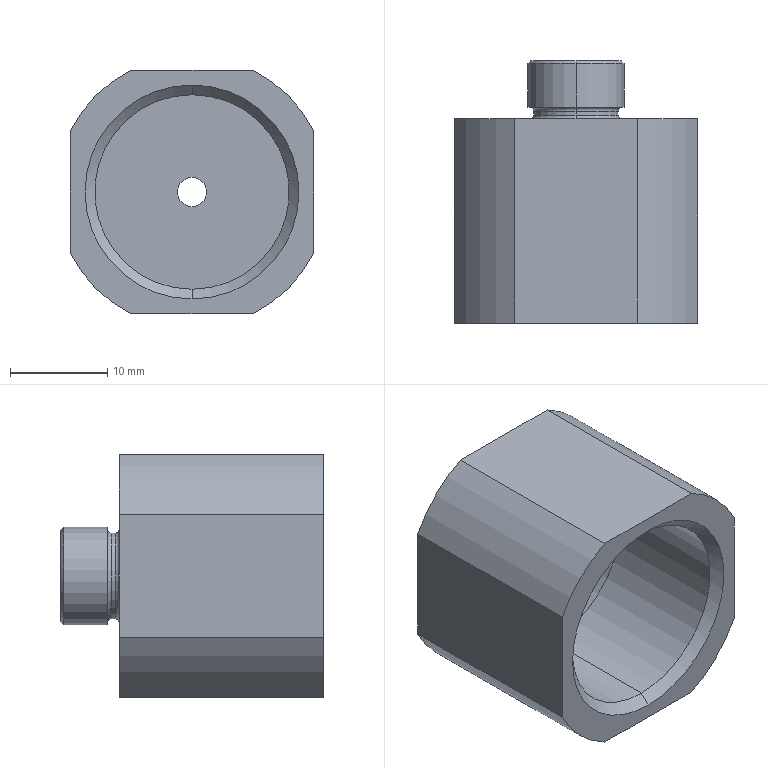Part | SolidWorks | features ICE 4, Chamfer 2, Fillet 1, Revolution 1 | 1 solid | 32 faces | box 25 x 27 x 25 mm | volume 6496 mm3 | cylinder 14 | plane 10 | cone 4 | torus 4 | commonest cylinder face diameters 28 x4 3 x2 8.8 x2 10 x2 20 x2 20.5 x2
STEP:
#1=CARTESIAN_POINT('',(0.,1.,10.));
#2=VERTEX_POINT('',#1);
#3=CARTESIAN_POINT('',(0.,1.,-10.));
#4=VERTEX_POINT('',#3);
#5=CARTESIAN_POINT('',(0.,1.,0.));
#6=DIRECTION('',(0.,-1.,0.));
#7=DIRECTION('',(0.,0.,-1.));
#8=AXIS2_PLACEMENT_3D('',#5,#6,#7);
#9=CIRCLE('',#8,10.);
#10=EDGE_CURVE('',#2,#4,#9,.T.);
#11=ORIENTED_EDGE('',*,*,#10,.F.);
#12=CARTESIAN_POINT('',(0.,0.,11.));
#13=VERTEX_POINT('',#12);
#14=CARTESIAN_POINT('',(0.,1.,10.));
#15=DIRECTION('',(0.,-0.7071,0.7071));
#16=VECTOR('',#15,1000.);
#17=LINE('',#14,#16);
#18=EDGE_CURVE('',#2,#13,#17,.T.);
#19=ORIENTED_EDGE('',*,*,#18,.T.);
#20=CARTESIAN_POINT('',(0.,0.,-11.));
#21=VERTEX_POINT('',#20);
#22=CARTESIAN_POINT('',(0.,0.,0.));
#23=DIRECTION('',(0.,1.,0.));
#24=DIRECTION('',(0.,0.,-1.));
#25=AXIS2_PLACEMENT_3D('',#22,#23,#24);
#26=CIRCLE('',#25,11.);
#27=EDGE_CURVE('',#21,#13,#26,.T.);
#28=ORIENTED_EDGE('',*,*,#27,.F.);
#29=CARTESIAN_POINT('',(0.,1.,-10.));
#30=DIRECTION('',(0.,-0.7071,-0.7071));
#31=VECTOR('',#30,1000.);
#32=LINE('',#29,#31);
#33=EDGE_CURVE('',#4,#21,#32,.T.);
#34=ORIENTED_EDGE('',*,*,#33,.F.);
#35=EDGE_LOOP('',(#11,#19,#28,#34));
#36=FACE_OUTER_BOUND('',#35,.T.);
#37=CARTESIAN_POINT('',(0.,1.,0.));
#38=DIRECTION('',(0.,-1.,0.));
#39=DIRECTION('',(0.,0.,-1.));
#40=AXIS2_PLACEMENT_3D('',#37,#38,#39);
#41=CONICAL_SURFACE('',#40,10.,0.7854);
#42=ADVANCED_FACE('',(#36),#41,.F.);
#43=CARTESIAN_POINT('',(0.,27.,4.7));
#44=VERTEX_POINT('',#43);
#45=CARTESIAN_POINT('',(0.,27.,-4.7));
#46=VERTEX_POINT('',#45);
#47=CARTESIAN_POINT('',(0.,27.,0.));
#48=DIRECTION('',(0.,1.,0.));
#49=DIRECTION('',(0.,0.,1.));
#50=AXIS2_PLACEMENT_3D('',#47,#48,#49);
#51=CIRCLE('',#50,4.7);
#52=EDGE_CURVE('',#44,#46,#51,.T.);
#53=ORIENTED_EDGE('',*,*,#52,.F.);
#54=CARTESIAN_POINT('',(0.,26.7,5.));
#55=VERTEX_POINT('',#54);
#56=CARTESIAN_POINT('',(0.,27.,4.7));
#57=DIRECTION('',(0.,-0.7071,0.7071));
#58=VECTOR('',#57,1000.);
#59=LINE('',#56,#58);
#60=EDGE_CURVE('',#44,#55,#59,.T.);
#61=ORIENTED_EDGE('',*,*,#60,.T.);
#62=CARTESIAN_POINT('',(0.,26.7,-5.));
#63=VERTEX_POINT('',#62);
#64=CARTESIAN_POINT('',(0.,26.7,0.));
#65=DIRECTION('',(0.,-1.,0.));
#66=DIRECTION('',(0.,0.,1.));
#67=AXIS2_PLACEMENT_3D('',#64,#65,#66);
#68=CIRCLE('',#67,5.);
#69=EDGE_CURVE('',#63,#55,#68,.T.);
#70=ORIENTED_EDGE('',*,*,#69,.F.);
#71=CARTESIAN_POINT('',(0.,27.,-4.7));
#72=DIRECTION('',(0.,-0.7071,-0.7071));
#73=VECTOR('',#72,1000.);
#74=LINE('',#71,#73);
#75=EDGE_CURVE('',#46,#63,#74,.T.);
#76=ORIENTED_EDGE('',*,*,#75,.F.);
#77=EDGE_LOOP('',(#53,#61,#70,#76));
#78=FACE_OUTER_BOUND('',#77,.T.);
#79=CARTESIAN_POINT('',(0.,27.,0.));
#80=DIRECTION('',(0.,-1.,0.));
#81=DIRECTION('',(0.,0.,-1.));
#82=AXIS2_PLACEMENT_3D('',#79,#80,#81);
#83=CONICAL_SURFACE('',#82,4.7,0.7854);
#84=ADVANCED_FACE('',(#78),#83,.T.);
#85=CARTESIAN_POINT('',(0.,27.,-1.5));
#86=VERTEX_POINT('',#85);
#87=CARTESIAN_POINT('',(0.,27.,1.5));
#88=VERTEX_POINT('',#87);
#89=CARTESIAN_POINT('',(0.,27.,0.));
#90=DIRECTION('',(0.,1.,0.));
#91=DIRECTION('',(0.,0.,1.));
#92=AXIS2_PLACEMENT_3D('',#89,#90,#91);
#93=CIRCLE('',#92,1.5);
#94=EDGE_CURVE('',#86,#88,#93,.T.);
#95=ORIENTED_EDGE('',*,*,#94,.T.);
#96=CARTESIAN_POINT('',(0.,18.,1.5));
#97=VERTEX_POINT('',#96);
#98=CARTESIAN_POINT('',(0.,108.,1.5));
#99=DIRECTION('',(0.,-1.,0.));
#100=VECTOR('',#99,1000.);
#101=LINE('',#98,#100);
#102=EDGE_CURVE('',#88,#97,#101,.T.);
#103=ORIENTED_EDGE('',*,*,#102,.T.);
#104=CARTESIAN_POINT('',(0.,18.,-1.5));
#105=VERTEX_POINT('',#104);
#106=CARTESIAN_POINT('',(0.,18.,0.));
#107=DIRECTION('',(0.,-1.,0.));
#108=DIRECTION('',(0.,0.,-1.));
#109=AXIS2_PLACEMENT_3D('',#106,#107,#108);
#110=CIRCLE('',#109,1.5);
#111=EDGE_CURVE('',#97,#105,#110,.T.);
#112=ORIENTED_EDGE('',*,*,#111,.T.);
#113=CARTESIAN_POINT('',(0.,108.,-1.5));
#114=DIRECTION('',(0.,-1.,0.));
#115=VECTOR('',#114,1000.);
#116=LINE('',#113,#115);
#117=EDGE_CURVE('',#86,#105,#116,.T.);
#118=ORIENTED_EDGE('',*,*,#117,.F.);
#119=EDGE_LOOP('',(#95,#103,#112,#118));
#120=FACE_OUTER_BOUND('',#119,.T.);
#121=CARTESIAN_POINT('',(0.,108.,0.));
#122=DIRECTION('',(0.,-1.,0.));
#123=DIRECTION('',(0.,0.,-1.));
#124=AXIS2_PLACEMENT_3D('',#121,#122,#123);
#125=CYLINDRICAL_SURFACE('',#124,1.5);
#126=ADVANCED_FACE('',(#120),#125,.F.);
#127=CARTESIAN_POINT('',(0.,18.,10.25));
#128=VERTEX_POINT('',#127);
#129=CARTESIAN_POINT('',(0.,18.,-10.25));
#130=VERTEX_POINT('',#129);
#131=CARTESIAN_POINT('',(0.,18.,0.));
#132=DIRECTION('',(0.,-1.,0.));
#133=DIRECTION('',(0.,0.,-1.));
#134=AXIS2_PLACEMENT_3D('',#131,#132,#133);
#135=CIRCLE('',#134,10.25);
#136=EDGE_CURVE('',#128,#130,#135,.T.);
#137=ORIENTED_EDGE('',*,*,#136,.F.);
#138=CARTESIAN_POINT('',(0.,14.,10.25));
#139=VERTEX_POINT('',#138);
#140=CARTESIAN_POINT('',(0.,18.,10.25));
#141=DIRECTION('',(0.,-1.,0.));
#142=VECTOR('',#141,1000.);
#143=LINE('',#140,#142);
#144=EDGE_CURVE('',#128,#139,#143,.T.);
#145=ORIENTED_EDGE('',*,*,#144,.T.);
#146=CARTESIAN_POINT('',(0.,14.,-10.25));
#147=VERTEX_POINT('',#146);
#148=CARTESIAN_POINT('',(0.,14.,0.));
#149=DIRECTION('',(0.,-1.,0.));
#150=DIRECTION('',(0.,0.,-1.));
#151=AXIS2_PLACEMENT_3D('',#148,#149,#150);
#152=CIRCLE('',#151,10.25);
#153=EDGE_CURVE('',#139,#147,#152,.T.);
#154=ORIENTED_EDGE('',*,*,#153,.T.);
#155=CARTESIAN_POINT('',(0.,18.,-10.25));
#156=DIRECTION('',(0.,-1.,0.));
#157=VECTOR('',#156,1000.);
#158=LINE('',#155,#157);
#159=EDGE_CURVE('',#130,#147,#158,.T.);
#160=ORIENTED_EDGE('',*,*,#159,.F.);
#161=EDGE_LOOP('',(#137,#145,#154,#160));
#162=FACE_OUTER_BOUND('',#161,.T.);
#163=CARTESIAN_POINT('',(0.,18.,0.));
#164=DIRECTION('',(0.,-1.,0.));
#165=DIRECTION('',(0.,0.,-1.));
#166=AXIS2_PLACEMENT_3D('',#163,#164,#165);
#167=CYLINDRICAL_SURFACE('',#166,10.25);
#168=ADVANCED_FACE('',(#162),#167,.F.);
#169=CARTESIAN_POINT('',(0.,14.,10.));
#170=VERTEX_POINT('',#169);
#171=CARTESIAN_POINT('',(0.,14.,-10.));
#172=VERTEX_POINT('',#171);
#173=CARTESIAN_POINT('',(0.,14.,0.));
#174=DIRECTION('',(0.,-1.,0.));
#175=DIRECTION('',(0.,0.,-1.));
#176=AXIS2_PLACEMENT_3D('',#173,#174,#175);
#177=CIRCLE('',#176,10.);
#178=EDGE_CURVE('',#170,#172,#177,.T.);
#179=ORIENTED_EDGE('',*,*,#178,.F.);
#180=CARTESIAN_POINT('',(0.,14.,10.));
#181=DIRECTION('',(0.,-1.,0.));
#182=VECTOR('',#181,1000.);
#183=LINE('',#180,#182);
#184=EDGE_CURVE('',#170,#2,#183,.T.);
#185=ORIENTED_EDGE('',*,*,#184,.T.);
#186=ORIENTED_EDGE('',*,*,#10,.T.);
#187=CARTESIAN_POINT('',(0.,14.,-10.));
#188=DIRECTION('',(0.,-1.,0.));
#189=VECTOR('',#188,1000.);
#190=LINE('',#187,#189);
#191=EDGE_CURVE('',#172,#4,#190,.T.);
#192=ORIENTED_EDGE('',*,*,#191,.F.);
#193=EDGE_LOOP('',(#179,#185,#186,#192));
#194=FACE_OUTER_BOUND('',#193,.T.);
#195=CARTESIAN_POINT('',(0.,14.,0.));
#196=DIRECTION('',(0.,-1.,0.));
#197=DIRECTION('',(0.,0.,-1.));
#198=AXIS2_PLACEMENT_3D('',#195,#196,#197);
#199=CYLINDRICAL_SURFACE('',#198,10.);
#200=ADVANCED_FACE('',(#194),#199,.F.);
#201=CARTESIAN_POINT('',(0.,21.4,-4.4));
#202=VERTEX_POINT('',#201);
#203=CARTESIAN_POINT('',(0.,21.4,4.4));
#204=VERTEX_POINT('',#203);
#205=CARTESIAN_POINT('',(0.,21.4,0.));
#206=DIRECTION('',(0.,1.,0.));
#207=DIRECTION('',(0.,0.,1.));
#208=AXIS2_PLACEMENT_3D('',#205,#206,#207);
#209=CIRCLE('',#208,4.4);
#210=EDGE_CURVE('',#202,#204,#209,.T.);
#211=ORIENTED_EDGE('',*,*,#210,.F.);
#212=CARTESIAN_POINT('',(0.,21.,-4.8));
#213=VERTEX_POINT('',#212);
#214=CARTESIAN_POINT('',(0.,21.4,-4.8));
#215=DIRECTION('',(1.,0.,0.));
#216=DIRECTION('',(0.,0.,-1.));
#217=AXIS2_PLACEMENT_3D('',#214,#215,#216);
#218=CIRCLE('',#217,0.4);
#219=EDGE_CURVE('',#202,#213,#218,.T.);
#220=ORIENTED_EDGE('',*,*,#219,.T.);
#221=CARTESIAN_POINT('',(0.,21.,4.8));
#222=VERTEX_POINT('',#221);
#223=CARTESIAN_POINT('',(0.,21.,0.));
#224=DIRECTION('',(0.,-1.,0.));
#225=DIRECTION('',(0.,0.,1.));
#226=AXIS2_PLACEMENT_3D('',#223,#224,#225);
#227=CIRCLE('',#226,4.8);
#228=EDGE_CURVE('',#222,#213,#227,.T.);
#229=ORIENTED_EDGE('',*,*,#228,.F.);
#230=CARTESIAN_POINT('',(0.,21.4,4.8));
#231=DIRECTION('',(-1.,0.,0.));
#232=DIRECTION('',(0.,0.,1.));
#233=AXIS2_PLACEMENT_3D('',#230,#231,#232);
#234=CIRCLE('',#233,0.4);
#235=EDGE_CURVE('',#204,#222,#234,.T.);
#236=ORIENTED_EDGE('',*,*,#235,.F.);
#237=EDGE_LOOP('',(#211,#220,#229,#236));
#238=FACE_OUTER_BOUND('',#237,.T.);
#239=CARTESIAN_POINT('',(0.,21.4,0.));
#240=DIRECTION('',(0.,1.,0.));
#241=DIRECTION('',(0.,0.,1.));
#242=AXIS2_PLACEMENT_3D('',#239,#240,#241);
#243=TOROIDAL_SURFACE('',#242,4.8,0.4);
#244=ADVANCED_FACE('',(#238),#243,.F.);
#245=CARTESIAN_POINT('',(0.,21.8,4.4));
#246=VERTEX_POINT('',#245);
#247=CARTESIAN_POINT('',(0.,21.8,-4.4));
#248=VERTEX_POINT('',#247);
#249=CARTESIAN_POINT('',(0.,21.8,0.));
#250=DIRECTION('',(0.,-1.,0.));
#251=DIRECTION('',(0.,0.,-1.));
#252=AXIS2_PLACEMENT_3D('',#249,#250,#251);
#253=CIRCLE('',#252,4.4);
#254=EDGE_CURVE('',#246,#248,#253,.T.);
#255=ORIENTED_EDGE('',*,*,#254,.F.);
#256=CARTESIAN_POINT('',(0.,22.2,4.8));
#257=VERTEX_POINT('',#256);
#258=CARTESIAN_POINT('',(0.,21.8,4.8));
#259=DIRECTION('',(1.,0.,0.));
#260=DIRECTION('',(0.,0.,-1.));
#261=AXIS2_PLACEMENT_3D('',#258,#259,#260);
#262=CIRCLE('',#261,0.4);
#263=EDGE_CURVE('',#246,#257,#262,.T.);
#264=ORIENTED_EDGE('',*,*,#263,.T.);
#265=CARTESIAN_POINT('',(0.,22.2,-4.8));
#266=VERTEX_POINT('',#265);
#267=CARTESIAN_POINT('',(0.,22.2,0.));
#268=DIRECTION('',(0.,1.,0.));
#269=DIRECTION('',(0.,0.,-1.));
#270=AXIS2_PLACEMENT_3D('',#267,#268,#269);
#271=CIRCLE('',#270,4.8);
#272=EDGE_CURVE('',#266,#257,#271,.T.);
#273=ORIENTED_EDGE('',*,*,#272,.F.);
#274=CARTESIAN_POINT('',(0.,21.8,-4.8));
#275=DIRECTION('',(-1.,0.,0.));
#276=DIRECTION('',(0.,0.,1.));
#277=AXIS2_PLACEMENT_3D('',#274,#275,#276);
#278=CIRCLE('',#277,0.4);
#279=EDGE_CURVE('',#248,#266,#278,.T.);
#280=ORIENTED_EDGE('',*,*,#279,.F.);
#281=EDGE_LOOP('',(#255,#264,#273,#280));
#282=FACE_OUTER_BOUND('',#281,.T.);
#283=CARTESIAN_POINT('',(0.,21.8,0.));
#284=DIRECTION('',(0.,-1.,0.));
#285=DIRECTION('',(0.,0.,-1.));
#286=AXIS2_PLACEMENT_3D('',#283,#284,#285);
#287=TOROIDAL_SURFACE('',#286,4.8,0.4);
#288=ADVANCED_FACE('',(#282),#287,.F.);
#289=CARTESIAN_POINT('',(0.,22.2,5.));
#290=VERTEX_POINT('',#289);
#291=CARTESIAN_POINT('',(0.,22.2,-5.));
#292=VERTEX_POINT('',#291);
#293=CARTESIAN_POINT('',(0.,22.2,0.));
#294=DIRECTION('',(0.,1.,0.));
#295=DIRECTION('',(0.,0.,1.));
#296=AXIS2_PLACEMENT_3D('',#293,#294,#295);
#297=CIRCLE('',#296,5.);
#298=EDGE_CURVE('',#290,#292,#297,.T.);
#299=ORIENTED_EDGE('',*,*,#298,.T.);
#300=CARTESIAN_POINT('',(0.,27.,-5.));
#301=DIRECTION('',(0.,1.,0.));
#302=VECTOR('',#301,1000.);
#303=LINE('',#300,#302);
#304=EDGE_CURVE('',#292,#63,#303,.T.);
#305=ORIENTED_EDGE('',*,*,#304,.T.);
#306=ORIENTED_EDGE('',*,*,#69,.T.);
#307=CARTESIAN_POINT('',(0.,27.,5.));
#308=DIRECTION('',(0.,1.,0.));
#309=VECTOR('',#308,1000.);
#310=LINE('',#307,#309);
#311=EDGE_CURVE('',#290,#55,#310,.T.);
#312=ORIENTED_EDGE('',*,*,#311,.F.);
#313=EDGE_LOOP('',(#299,#305,#306,#312));
#314=FACE_OUTER_BOUND('',#313,.T.);
#315=CARTESIAN_POINT('',(0.,27.,0.));
#316=DIRECTION('',(0.,1.,0.));
#317=DIRECTION('',(0.,0.,1.));
#318=AXIS2_PLACEMENT_3D('',#315,#316,#317);
#319=CYLINDRICAL_SURFACE('',#318,5.);
#320=ADVANCED_FACE('',(#314),#319,.T.);
#321=CARTESIAN_POINT('',(0.,21.4,0.));
#322=DIRECTION('',(0.,1.,0.));
#323=DIRECTION('',(0.,0.,1.));
#324=AXIS2_PLACEMENT_3D('',#321,#322,#323);
#325=CIRCLE('',#324,4.4);
#326=EDGE_CURVE('',#204,#202,#325,.T.);
#327=ORIENTED_EDGE('',*,*,#326,.T.);
#328=CARTESIAN_POINT('',(0.,27.,-4.4));
#329=DIRECTION('',(0.,1.,0.));
#330=VECTOR('',#329,1000.);
#331=LINE('',#328,#330);
#332=EDGE_CURVE('',#202,#248,#331,.T.);
#333=ORIENTED_EDGE('',*,*,#332,.T.);
#334=CARTESIAN_POINT('',(0.,21.8,0.));
#335=DIRECTION('',(0.,-1.,0.));
#336=DIRECTION('',(0.,0.,-1.));
#337=AXIS2_PLACEMENT_3D('',#334,#335,#336);
#338=CIRCLE('',#337,4.4);
#339=EDGE_CURVE('',#248,#246,#338,.T.);
#340=ORIENTED_EDGE('',*,*,#339,.T.);
#341=CARTESIAN_POINT('',(0.,27.,4.4));
#342=DIRECTION('',(0.,1.,0.));
#343=VECTOR('',#342,1000.);
#344=LINE('',#341,#343);
#345=EDGE_CURVE('',#204,#246,#344,.T.);
#346=ORIENTED_EDGE('',*,*,#345,.F.);
#347=EDGE_LOOP('',(#327,#333,#340,#346));
#348=FACE_OUTER_BOUND('',#347,.T.);
#349=CARTESIAN_POINT('',(0.,27.,0.));
#350=DIRECTION('',(0.,1.,0.));
#351=DIRECTION('',(0.,0.,1.));
#352=AXIS2_PLACEMENT_3D('',#349,#350,#351);
#353=CYLINDRICAL_SURFACE('',#352,4.4);
#354=ADVANCED_FACE('',(#348),#353,.T.);
#355=ORIENTED_EDGE('',*,*,#27,.T.);
#356=CARTESIAN_POINT('',(0.,0.,0.));
#357=DIRECTION('',(0.,1.,0.));
#358=DIRECTION('',(0.,0.,-1.));
#359=AXIS2_PLACEMENT_3D('',#356,#357,#358);
#360=CIRCLE('',#359,11.);
#361=EDGE_CURVE('',#13,#21,#360,.T.);
#362=ORIENTED_EDGE('',*,*,#361,.T.);
#363=EDGE_LOOP('',(#355,#362));
#364=FACE_BOUND('',#363,.T.);
#365=CARTESIAN_POINT('',(-12.5,0.,6.305));
#366=VERTEX_POINT('',#365);
#367=CARTESIAN_POINT('',(-6.305,0.,12.5));
#368=VERTEX_POINT('',#367);
#369=CARTESIAN_POINT('',(0.,0.,0.));
#370=DIRECTION('',(0.,1.,0.));
#371=DIRECTION('',(0.,0.,1.));
#372=AXIS2_PLACEMENT_3D('',#369,#370,#371);
#373=CIRCLE('',#372,14.);
#374=EDGE_CURVE('',#366,#368,#373,.T.);
#375=ORIENTED_EDGE('',*,*,#374,.F.);
#376=CARTESIAN_POINT('',(-12.5,0.,-6.305));
#377=VERTEX_POINT('',#376);
#378=CARTESIAN_POINT('',(-12.5,0.,0.));
#379=DIRECTION('',(0.,0.,-1.));
#380=VECTOR('',#379,1000.);
#381=LINE('',#378,#380);
#382=EDGE_CURVE('',#366,#377,#381,.T.);
#383=ORIENTED_EDGE('',*,*,#382,.T.);
#384=CARTESIAN_POINT('',(-6.305,0.,-12.5));
#385=VERTEX_POINT('',#384);
#386=CARTESIAN_POINT('',(0.,0.,0.));
#387=DIRECTION('',(0.,1.,0.));
#388=DIRECTION('',(0.,0.,1.));
#389=AXIS2_PLACEMENT_3D('',#386,#387,#388);
#390=CIRCLE('',#389,14.);
#391=EDGE_CURVE('',#385,#377,#390,.T.);
#392=ORIENTED_EDGE('',*,*,#391,.F.);
#393=CARTESIAN_POINT('',(6.305,0.,-12.5));
#394=VERTEX_POINT('',#393);
#395=CARTESIAN_POINT('',(0.,0.,-12.5));
#396=DIRECTION('',(1.,0.,0.));
#397=VECTOR('',#396,1000.);
#398=LINE('',#395,#397);
#399=EDGE_CURVE('',#385,#394,#398,.T.);
#400=ORIENTED_EDGE('',*,*,#399,.T.);
#401=CARTESIAN_POINT('',(12.5,0.,-6.305));
#402=VERTEX_POINT('',#401);
#403=CARTESIAN_POINT('',(0.,0.,0.));
#404=DIRECTION('',(0.,1.,0.));
#405=DIRECTION('',(0.,0.,1.));
#406=AXIS2_PLACEMENT_3D('',#403,#404,#405);
#407=CIRCLE('',#406,14.);
#408=EDGE_CURVE('',#402,#394,#407,.T.);
#409=ORIENTED_EDGE('',*,*,#408,.F.);
#410=CARTESIAN_POINT('',(12.5,0.,6.305));
#411=VERTEX_POINT('',#410);
#412=CARTESIAN_POINT('',(12.5,0.,0.));
#413=DIRECTION('',(0.,0.,1.));
#414=VECTOR('',#413,1000.);
#415=LINE('',#412,#414);
#416=EDGE_CURVE('',#402,#411,#415,.T.);
#417=ORIENTED_EDGE('',*,*,#416,.T.);
#418=CARTESIAN_POINT('',(6.305,0.,12.5));
#419=VERTEX_POINT('',#418);
#420=CARTESIAN_POINT('',(0.,0.,0.));
#421=DIRECTION('',(0.,1.,0.));
#422=DIRECTION('',(0.,0.,1.));
#423=AXIS2_PLACEMENT_3D('',#420,#421,#422);
#424=CIRCLE('',#423,14.);
#425=EDGE_CURVE('',#419,#411,#424,.T.);
#426=ORIENTED_EDGE('',*,*,#425,.F.);
#427=CARTESIAN_POINT('',(0.,0.,12.5));
#428=DIRECTION('',(-1.,0.,0.));
#429=VECTOR('',#428,1000.);
#430=LINE('',#427,#429);
#431=EDGE_CURVE('',#419,#368,#430,.T.);
#432=ORIENTED_EDGE('',*,*,#431,.T.);
#433=EDGE_LOOP('',(#375,#383,#392,#400,#409,#417,#426,#432));
#434=FACE_OUTER_BOUND('',#433,.T.);
#435=CARTESIAN_POINT('',(0.,0.,0.));
#436=DIRECTION('',(0.,-1.,0.));
#437=DIRECTION('',(0.,0.,-1.));
#438=AXIS2_PLACEMENT_3D('',#435,#436,#437);
#439=PLANE('',#438);
#440=ADVANCED_FACE('',(#364,#434),#439,.T.);
#441=CARTESIAN_POINT('',(-12.5,21.,6.305));
#442=VERTEX_POINT('',#441);
#443=CARTESIAN_POINT('',(-6.305,21.,12.5));
#444=VERTEX_POINT('',#443);
#445=CARTESIAN_POINT('',(0.,21.,0.));
#446=DIRECTION('',(0.,1.,0.));
#447=DIRECTION('',(0.,0.,1.));
#448=AXIS2_PLACEMENT_3D('',#445,#446,#447);
#449=CIRCLE('',#448,14.);
#450=EDGE_CURVE('',#442,#444,#449,.T.);
#451=ORIENTED_EDGE('',*,*,#450,.F.);
#452=CARTESIAN_POINT('',(-12.5,27.,6.305));
#453=DIRECTION('',(0.,-1.,0.));
#454=VECTOR('',#453,1000.);
#455=LINE('',#452,#454);
#456=EDGE_CURVE('',#442,#366,#455,.T.);
#457=ORIENTED_EDGE('',*,*,#456,.T.);
#458=ORIENTED_EDGE('',*,*,#374,.T.);
#459=CARTESIAN_POINT('',(-6.305,27.,12.5));
#460=DIRECTION('',(0.,1.,0.));
#461=VECTOR('',#460,1000.);
#462=LINE('',#459,#461);
#463=EDGE_CURVE('',#368,#444,#462,.T.);
#464=ORIENTED_EDGE('',*,*,#463,.T.);
#465=EDGE_LOOP('',(#451,#457,#458,#464));
#466=FACE_OUTER_BOUND('',#465,.T.);
#467=CARTESIAN_POINT('',(0.,27.,0.));
#468=DIRECTION('',(0.,1.,0.));
#469=DIRECTION('',(0.,0.,1.));
#470=AXIS2_PLACEMENT_3D('',#467,#468,#469);
#471=CYLINDRICAL_SURFACE('',#470,14.);
#472=ADVANCED_FACE('',(#466),#471,.T.);
#473=ORIENTED_EDGE('',*,*,#391,.T.);
#474=CARTESIAN_POINT('',(-12.5,21.,-6.305));
#475=VERTEX_POINT('',#474);
#476=CARTESIAN_POINT('',(-12.5,27.,-6.305));
#477=DIRECTION('',(0.,1.,0.));
#478=VECTOR('',#477,1000.);
#479=LINE('',#476,#478);
#480=EDGE_CURVE('',#377,#475,#479,.T.);
#481=ORIENTED_EDGE('',*,*,#480,.T.);
#482=CARTESIAN_POINT('',(-6.305,21.,-12.5));
#483=VERTEX_POINT('',#482);
#484=CARTESIAN_POINT('',(0.,21.,0.));
#485=DIRECTION('',(0.,1.,0.));
#486=DIRECTION('',(0.,0.,1.));
#487=AXIS2_PLACEMENT_3D('',#484,#485,#486);
#488=CIRCLE('',#487,14.);
#489=EDGE_CURVE('',#483,#475,#488,.T.);
#490=ORIENTED_EDGE('',*,*,#489,.F.);
#491=CARTESIAN_POINT('',(-6.305,27.,-12.5));
#492=DIRECTION('',(0.,-1.,0.));
#493=VECTOR('',#492,1000.);
#494=LINE('',#491,#493);
#495=EDGE_CURVE('',#483,#385,#494,.T.);
#496=ORIENTED_EDGE('',*,*,#495,.T.);
#497=EDGE_LOOP('',(#473,#481,#490,#496));
#498=FACE_OUTER_BOUND('',#497,.T.);
#499=CARTESIAN_POINT('',(0.,27.,0.));
#500=DIRECTION('',(0.,1.,0.));
#501=DIRECTION('',(0.,0.,1.));
#502=AXIS2_PLACEMENT_3D('',#499,#500,#501);
#503=CYLINDRICAL_SURFACE('',#502,14.);
#504=ADVANCED_FACE('',(#498),#503,.T.);
#505=ORIENTED_EDGE('',*,*,#408,.T.);
#506=CARTESIAN_POINT('',(6.305,21.,-12.5));
#507=VERTEX_POINT('',#506);
#508=CARTESIAN_POINT('',(6.305,27.,-12.5));
#509=DIRECTION('',(0.,1.,0.));
#510=VECTOR('',#509,1000.);
#511=LINE('',#508,#510);
#512=EDGE_CURVE('',#394,#507,#511,.T.);
#513=ORIENTED_EDGE('',*,*,#512,.T.);
#514=CARTESIAN_POINT('',(12.5,21.,-6.305));
#515=VERTEX_POINT('',#514);
#516=CARTESIAN_POINT('',(0.,21.,0.));
#517=DIRECTION('',(0.,1.,0.));
#518=DIRECTION('',(0.,0.,1.));
#519=AXIS2_PLACEMENT_3D('',#516,#517,#518);
#520=CIRCLE('',#519,14.);
#521=EDGE_CURVE('',#515,#507,#520,.T.);
#522=ORIENTED_EDGE('',*,*,#521,.F.);
#523=CARTESIAN_POINT('',(12.5,27.,-6.305));
#524=DIRECTION('',(0.,-1.,0.));
#525=VECTOR('',#524,1000.);
#526=LINE('',#523,#525);
#527=EDGE_CURVE('',#515,#402,#526,.T.);
#528=ORIENTED_EDGE('',*,*,#527,.T.);
#529=EDGE_LOOP('',(#505,#513,#522,#528));
#530=FACE_OUTER_BOUND('',#529,.T.);
#531=CARTESIAN_POINT('',(0.,27.,0.));
#532=DIRECTION('',(0.,1.,0.));
#533=DIRECTION('',(0.,0.,1.));
#534=AXIS2_PLACEMENT_3D('',#531,#532,#533);
#535=CYLINDRICAL_SURFACE('',#534,14.);
#536=ADVANCED_FACE('',(#530),#535,.T.);
#537=ORIENTED_EDGE('',*,*,#425,.T.);
#538=CARTESIAN_POINT('',(12.5,21.,6.305));
#539=VERTEX_POINT('',#538);
#540=CARTESIAN_POINT('',(12.5,27.,6.305));
#541=DIRECTION('',(0.,1.,0.));
#542=VECTOR('',#541,1000.);
#543=LINE('',#540,#542);
#544=EDGE_CURVE('',#411,#539,#543,.T.);
#545=ORIENTED_EDGE('',*,*,#544,.T.);
#546=CARTESIAN_POINT('',(6.305,21.,12.5));
#547=VERTEX_POINT('',#546);
#548=CARTESIAN_POINT('',(0.,21.,0.));
#549=DIRECTION('',(0.,1.,0.));
#550=DIRECTION('',(0.,0.,1.));
#551=AXIS2_PLACEMENT_3D('',#548,#549,#550);
#552=CIRCLE('',#551,14.);
#553=EDGE_CURVE('',#547,#539,#552,.T.);
#554=ORIENTED_EDGE('',*,*,#553,.F.);
#555=CARTESIAN_POINT('',(6.305,27.,12.5));
#556=DIRECTION('',(0.,-1.,0.));
#557=VECTOR('',#556,1000.);
#558=LINE('',#555,#557);
#559=EDGE_CURVE('',#547,#419,#558,.T.);
#560=ORIENTED_EDGE('',*,*,#559,.T.);
#561=EDGE_LOOP('',(#537,#545,#554,#560));
#562=FACE_OUTER_BOUND('',#561,.T.);
#563=CARTESIAN_POINT('',(0.,27.,0.));
#564=DIRECTION('',(0.,1.,0.));
#565=DIRECTION('',(0.,0.,1.));
#566=AXIS2_PLACEMENT_3D('',#563,#564,#565);
#567=CYLINDRICAL_SURFACE('',#566,14.);
#568=ADVANCED_FACE('',(#562),#567,.T.);
#569=ORIENTED_EDGE('',*,*,#228,.T.);
#570=CARTESIAN_POINT('',(0.,21.,0.));
#571=DIRECTION('',(0.,-1.,0.));
#572=DIRECTION('',(0.,0.,1.));
#573=AXIS2_PLACEMENT_3D('',#570,#571,#572);
#574=CIRCLE('',#573,4.8);
#575=EDGE_CURVE('',#213,#222,#574,.T.);
#576=ORIENTED_EDGE('',*,*,#575,.T.);
#577=EDGE_LOOP('',(#569,#576));
#578=FACE_BOUND('',#577,.T.);
#579=ORIENTED_EDGE('',*,*,#489,.T.);
#580=CARTESIAN_POINT('',(-12.5,21.,0.));
#581=DIRECTION('',(0.,0.,1.));
#582=VECTOR('',#581,1000.);
#583=LINE('',#580,#582);
#584=EDGE_CURVE('',#475,#442,#583,.T.);
#585=ORIENTED_EDGE('',*,*,#584,.T.);
#586=ORIENTED_EDGE('',*,*,#450,.T.);
#587=CARTESIAN_POINT('',(-14.,21.,12.5));
#588=DIRECTION('',(1.,0.,0.));
#589=VECTOR('',#588,1000.);
#590=LINE('',#587,#589);
#591=EDGE_CURVE('',#444,#547,#590,.T.);
#592=ORIENTED_EDGE('',*,*,#591,.T.);
#593=ORIENTED_EDGE('',*,*,#553,.T.);
#594=CARTESIAN_POINT('',(12.5,21.,0.));
#595=DIRECTION('',(0.,0.,-1.));
#596=VECTOR('',#595,1000.);
#597=LINE('',#594,#596);
#598=EDGE_CURVE('',#539,#515,#597,.T.);
#599=ORIENTED_EDGE('',*,*,#598,.T.);
#600=ORIENTED_EDGE('',*,*,#521,.T.);
#601=CARTESIAN_POINT('',(-14.,21.,-12.5));
#602=DIRECTION('',(-1.,0.,0.));
#603=VECTOR('',#602,1000.);
#604=LINE('',#601,#603);
#605=EDGE_CURVE('',#507,#483,#604,.T.);
#606=ORIENTED_EDGE('',*,*,#605,.T.);
#607=EDGE_LOOP('',(#579,#585,#586,#592,#593,#599,#600,#606));
#608=FACE_OUTER_BOUND('',#607,.T.);
#609=CARTESIAN_POINT('',(-14.,21.,0.));
#610=DIRECTION('',(0.,1.,0.));
#611=DIRECTION('',(0.,0.,1.));
#612=AXIS2_PLACEMENT_3D('',#609,#610,#611);
#613=PLANE('',#612);
#614=ADVANCED_FACE('',(#578,#608),#613,.T.);
#615=ORIENTED_EDGE('',*,*,#332,.F.);
#616=ORIENTED_EDGE('',*,*,#210,.T.);
#617=ORIENTED_EDGE('',*,*,#345,.T.);
#618=ORIENTED_EDGE('',*,*,#254,.T.);
#619=EDGE_LOOP('',(#615,#616,#617,#618));
#620=FACE_OUTER_BOUND('',#619,.T.);
#621=CARTESIAN_POINT('',(0.,27.,0.));
#622=DIRECTION('',(0.,1.,0.));
#623=DIRECTION('',(0.,0.,1.));
#624=AXIS2_PLACEMENT_3D('',#621,#622,#623);
#625=CYLINDRICAL_SURFACE('',#624,4.4);
#626=ADVANCED_FACE('',(#620),#625,.T.);
#627=ORIENTED_EDGE('',*,*,#272,.T.);
#628=CARTESIAN_POINT('',(0.,22.2,0.));
#629=DIRECTION('',(0.,1.,0.));
#630=DIRECTION('',(0.,0.,-1.));
#631=AXIS2_PLACEMENT_3D('',#628,#629,#630);
#632=CIRCLE('',#631,4.8);
#633=EDGE_CURVE('',#257,#266,#632,.T.);
#634=ORIENTED_EDGE('',*,*,#633,.T.);
#635=EDGE_LOOP('',(#627,#634));
#636=FACE_BOUND('',#635,.T.);
#637=ORIENTED_EDGE('',*,*,#298,.F.);
#638=CARTESIAN_POINT('',(0.,22.2,0.));
#639=DIRECTION('',(0.,1.,0.));
#640=DIRECTION('',(0.,0.,1.));
#641=AXIS2_PLACEMENT_3D('',#638,#639,#640);
#642=CIRCLE('',#641,5.);
#643=EDGE_CURVE('',#292,#290,#642,.T.);
#644=ORIENTED_EDGE('',*,*,#643,.F.);
#645=EDGE_LOOP('',(#637,#644));
#646=FACE_OUTER_BOUND('',#645,.T.);
#647=CARTESIAN_POINT('',(-4.4,22.2,0.));
#648=DIRECTION('',(0.,-1.,0.));
#649=DIRECTION('',(0.,0.,-1.));
#650=AXIS2_PLACEMENT_3D('',#647,#648,#649);
#651=PLANE('',#650);
#652=ADVANCED_FACE('',(#636,#646),#651,.T.);
#653=ORIENTED_EDGE('',*,*,#304,.F.);
#654=ORIENTED_EDGE('',*,*,#643,.T.);
#655=ORIENTED_EDGE('',*,*,#311,.T.);
#656=CARTESIAN_POINT('',(0.,26.7,0.));
#657=DIRECTION('',(0.,-1.,0.));
#658=DIRECTION('',(0.,0.,1.));
#659=AXIS2_PLACEMENT_3D('',#656,#657,#658);
#660=CIRCLE('',#659,5.);
#661=EDGE_CURVE('',#55,#63,#660,.T.);
#662=ORIENTED_EDGE('',*,*,#661,.T.);
#663=EDGE_LOOP('',(#653,#654,#655,#662));
#664=FACE_OUTER_BOUND('',#663,.T.);
#665=CARTESIAN_POINT('',(0.,27.,0.));
#666=DIRECTION('',(0.,1.,0.));
#667=DIRECTION('',(0.,0.,1.));
#668=AXIS2_PLACEMENT_3D('',#665,#666,#667);
#669=CYLINDRICAL_SURFACE('',#668,5.);
#670=ADVANCED_FACE('',(#664),#669,.T.);
#671=CARTESIAN_POINT('',(0.,27.,0.));
#672=DIRECTION('',(0.,1.,0.));
#673=DIRECTION('',(0.,0.,1.));
#674=AXIS2_PLACEMENT_3D('',#671,#672,#673);
#675=CIRCLE('',#674,4.7);
#676=EDGE_CURVE('',#46,#44,#675,.T.);
#677=ORIENTED_EDGE('',*,*,#676,.T.);
#678=ORIENTED_EDGE('',*,*,#52,.T.);
#679=EDGE_LOOP('',(#677,#678));
#680=FACE_OUTER_BOUND('',#679,.T.);
#681=ORIENTED_EDGE('',*,*,#94,.F.);
#682=CARTESIAN_POINT('',(0.,27.,0.));
#683=DIRECTION('',(0.,1.,0.));
#684=DIRECTION('',(0.,0.,1.));
#685=AXIS2_PLACEMENT_3D('',#682,#683,#684);
#686=CIRCLE('',#685,1.5);
#687=EDGE_CURVE('',#88,#86,#686,.T.);
#688=ORIENTED_EDGE('',*,*,#687,.F.);
#689=EDGE_LOOP('',(#681,#688));
#690=FACE_BOUND('',#689,.T.);
#691=CARTESIAN_POINT('',(-5.,27.,0.));
#692=DIRECTION('',(0.,1.,0.));
#693=DIRECTION('',(0.,0.,1.));
#694=AXIS2_PLACEMENT_3D('',#691,#692,#693);
#695=PLANE('',#694);
#696=ADVANCED_FACE('',(#680,#690),#695,.T.);
#697=ORIENTED_EDGE('',*,*,#263,.F.);
#698=ORIENTED_EDGE('',*,*,#339,.F.);
#699=ORIENTED_EDGE('',*,*,#279,.T.);
#700=ORIENTED_EDGE('',*,*,#633,.F.);
#701=EDGE_LOOP('',(#697,#698,#699,#700));
#702=FACE_OUTER_BOUND('',#701,.T.);
#703=CARTESIAN_POINT('',(0.,21.8,0.));
#704=DIRECTION('',(0.,-1.,0.));
#705=DIRECTION('',(0.,0.,-1.));
#706=AXIS2_PLACEMENT_3D('',#703,#704,#705);
#707=TOROIDAL_SURFACE('',#706,4.8,0.4);
#708=ADVANCED_FACE('',(#702),#707,.F.);
#709=ORIENTED_EDGE('',*,*,#219,.F.);
#710=ORIENTED_EDGE('',*,*,#326,.F.);
#711=ORIENTED_EDGE('',*,*,#235,.T.);
#712=ORIENTED_EDGE('',*,*,#575,.F.);
#713=EDGE_LOOP('',(#709,#710,#711,#712));
#714=FACE_OUTER_BOUND('',#713,.T.);
#715=CARTESIAN_POINT('',(0.,21.4,0.));
#716=DIRECTION('',(0.,1.,0.));
#717=DIRECTION('',(0.,0.,1.));
#718=AXIS2_PLACEMENT_3D('',#715,#716,#717);
#719=TOROIDAL_SURFACE('',#718,4.8,0.4);
#720=ADVANCED_FACE('',(#714),#719,.F.);
#721=ORIENTED_EDGE('',*,*,#184,.F.);
#722=CARTESIAN_POINT('',(0.,14.,0.));
#723=DIRECTION('',(0.,-1.,0.));
#724=DIRECTION('',(0.,0.,-1.));
#725=AXIS2_PLACEMENT_3D('',#722,#723,#724);
#726=CIRCLE('',#725,10.);
#727=EDGE_CURVE('',#172,#170,#726,.T.);
#728=ORIENTED_EDGE('',*,*,#727,.F.);
#729=ORIENTED_EDGE('',*,*,#191,.T.);
#730=CARTESIAN_POINT('',(0.,1.,0.));
#731=DIRECTION('',(0.,-1.,0.));
#732=DIRECTION('',(0.,0.,-1.));
#733=AXIS2_PLACEMENT_3D('',#730,#731,#732);
#734=CIRCLE('',#733,10.);
#735=EDGE_CURVE('',#4,#2,#734,.T.);
#736=ORIENTED_EDGE('',*,*,#735,.T.);
#737=EDGE_LOOP('',(#721,#728,#729,#736));
#738=FACE_OUTER_BOUND('',#737,.T.);
#739=CARTESIAN_POINT('',(0.,14.,0.));
#740=DIRECTION('',(0.,-1.,0.));
#741=DIRECTION('',(0.,0.,-1.));
#742=AXIS2_PLACEMENT_3D('',#739,#740,#741);
#743=CYLINDRICAL_SURFACE('',#742,10.);
#744=ADVANCED_FACE('',(#738),#743,.F.);
#745=ORIENTED_EDGE('',*,*,#144,.F.);
#746=CARTESIAN_POINT('',(0.,18.,0.));
#747=DIRECTION('',(0.,-1.,0.));
#748=DIRECTION('',(0.,0.,-1.));
#749=AXIS2_PLACEMENT_3D('',#746,#747,#748);
#750=CIRCLE('',#749,10.25);
#751=EDGE_CURVE('',#130,#128,#750,.T.);
#752=ORIENTED_EDGE('',*,*,#751,.F.);
#753=ORIENTED_EDGE('',*,*,#159,.T.);
#754=CARTESIAN_POINT('',(0.,14.,0.));
#755=DIRECTION('',(0.,-1.,0.));
#756=DIRECTION('',(0.,0.,-1.));
#757=AXIS2_PLACEMENT_3D('',#754,#755,#756);
#758=CIRCLE('',#757,10.25);
#759=EDGE_CURVE('',#147,#139,#758,.T.);
#760=ORIENTED_EDGE('',*,*,#759,.T.);
#761=EDGE_LOOP('',(#745,#752,#753,#760));
#762=FACE_OUTER_BOUND('',#761,.T.);
#763=CARTESIAN_POINT('',(0.,18.,0.));
#764=DIRECTION('',(0.,-1.,0.));
#765=DIRECTION('',(0.,0.,-1.));
#766=AXIS2_PLACEMENT_3D('',#763,#764,#765);
#767=CYLINDRICAL_SURFACE('',#766,10.25);
#768=ADVANCED_FACE('',(#762),#767,.F.);
#769=CARTESIAN_POINT('',(0.,18.,0.));
#770=DIRECTION('',(0.,-1.,0.));
#771=DIRECTION('',(0.,0.,-1.));
#772=AXIS2_PLACEMENT_3D('',#769,#770,#771);
#773=CIRCLE('',#772,1.5);
#774=EDGE_CURVE('',#105,#97,#773,.T.);
#775=ORIENTED_EDGE('',*,*,#774,.F.);
#776=ORIENTED_EDGE('',*,*,#111,.F.);
#777=EDGE_LOOP('',(#775,#776));
#778=FACE_BOUND('',#777,.T.);
#779=ORIENTED_EDGE('',*,*,#751,.T.);
#780=ORIENTED_EDGE('',*,*,#136,.T.);
#781=EDGE_LOOP('',(#779,#780));
#782=FACE_OUTER_BOUND('',#781,.T.);
#783=CARTESIAN_POINT('',(0.,18.,0.));
#784=DIRECTION('',(0.,-1.,0.));
#785=DIRECTION('',(0.,0.,-1.));
#786=AXIS2_PLACEMENT_3D('',#783,#784,#785);
#787=PLANE('',#786);
#788=ADVANCED_FACE('',(#778,#782),#787,.T.);
#789=ORIENTED_EDGE('',*,*,#727,.T.);
#790=ORIENTED_EDGE('',*,*,#178,.T.);
#791=EDGE_LOOP('',(#789,#790));
#792=FACE_BOUND('',#791,.T.);
#793=ORIENTED_EDGE('',*,*,#759,.F.);
#794=ORIENTED_EDGE('',*,*,#153,.F.);
#795=EDGE_LOOP('',(#793,#794));
#796=FACE_OUTER_BOUND('',#795,.T.);
#797=CARTESIAN_POINT('',(0.,14.,0.));
#798=DIRECTION('',(0.,-1.,0.));
#799=DIRECTION('',(0.,0.,-1.));
#800=AXIS2_PLACEMENT_3D('',#797,#798,#799);
#801=PLANE('',#800);
#802=ADVANCED_FACE('',(#792,#796),#801,.F.);
#803=ORIENTED_EDGE('',*,*,#102,.F.);
#804=ORIENTED_EDGE('',*,*,#687,.T.);
#805=ORIENTED_EDGE('',*,*,#117,.T.);
#806=ORIENTED_EDGE('',*,*,#774,.T.);
#807=EDGE_LOOP('',(#803,#804,#805,#806));
#808=FACE_OUTER_BOUND('',#807,.T.);
#809=CARTESIAN_POINT('',(0.,108.,0.));
#810=DIRECTION('',(0.,-1.,0.));
#811=DIRECTION('',(0.,0.,-1.));
#812=AXIS2_PLACEMENT_3D('',#809,#810,#811);
#813=CYLINDRICAL_SURFACE('',#812,1.5);
#814=ADVANCED_FACE('',(#808),#813,.F.);
#815=ORIENTED_EDGE('',*,*,#60,.F.);
#816=ORIENTED_EDGE('',*,*,#676,.F.);
#817=ORIENTED_EDGE('',*,*,#75,.T.);
#818=ORIENTED_EDGE('',*,*,#661,.F.);
#819=EDGE_LOOP('',(#815,#816,#817,#818));
#820=FACE_OUTER_BOUND('',#819,.T.);
#821=CARTESIAN_POINT('',(0.,27.,0.));
#822=DIRECTION('',(0.,-1.,0.));
#823=DIRECTION('',(0.,0.,-1.));
#824=AXIS2_PLACEMENT_3D('',#821,#822,#823);
#825=CONICAL_SURFACE('',#824,4.7,0.7854);
#826=ADVANCED_FACE('',(#820),#825,.T.);
#827=ORIENTED_EDGE('',*,*,#18,.F.);
#828=ORIENTED_EDGE('',*,*,#735,.F.);
#829=ORIENTED_EDGE('',*,*,#33,.T.);
#830=ORIENTED_EDGE('',*,*,#361,.F.);
#831=EDGE_LOOP('',(#827,#828,#829,#830));
#832=FACE_OUTER_BOUND('',#831,.T.);
#833=CARTESIAN_POINT('',(0.,1.,0.));
#834=DIRECTION('',(0.,-1.,0.));
#835=DIRECTION('',(0.,0.,-1.));
#836=AXIS2_PLACEMENT_3D('',#833,#834,#835);
#837=CONICAL_SURFACE('',#836,10.,0.7854);
#838=ADVANCED_FACE('',(#832),#837,.F.);
#839=ORIENTED_EDGE('',*,*,#591,.F.);
#840=ORIENTED_EDGE('',*,*,#463,.F.);
#841=ORIENTED_EDGE('',*,*,#431,.F.);
#842=ORIENTED_EDGE('',*,*,#559,.F.);
#843=EDGE_LOOP('',(#839,#840,#841,#842));
#844=FACE_OUTER_BOUND('',#843,.T.);
#845=CARTESIAN_POINT('',(12.5,-69.,12.5));
#846=DIRECTION('',(0.,0.,1.));
#847=DIRECTION('',(1.,0.,0.));
#848=AXIS2_PLACEMENT_3D('',#845,#846,#847);
#849=PLANE('',#848);
#850=ADVANCED_FACE('',(#844),#849,.T.);
#851=ORIENTED_EDGE('',*,*,#598,.F.);
#852=ORIENTED_EDGE('',*,*,#544,.F.);
#853=ORIENTED_EDGE('',*,*,#416,.F.);
#854=ORIENTED_EDGE('',*,*,#527,.F.);
#855=EDGE_LOOP('',(#851,#852,#853,#854));
#856=FACE_OUTER_BOUND('',#855,.T.);
#857=CARTESIAN_POINT('',(12.5,-69.,12.5));
#858=DIRECTION('',(1.,0.,0.));
#859=DIRECTION('',(0.,0.,-1.));
#860=AXIS2_PLACEMENT_3D('',#857,#858,#859);
#861=PLANE('',#860);
#862=ADVANCED_FACE('',(#856),#861,.T.);
#863=ORIENTED_EDGE('',*,*,#605,.F.);
#864=ORIENTED_EDGE('',*,*,#512,.F.);
#865=ORIENTED_EDGE('',*,*,#399,.F.);
#866=ORIENTED_EDGE('',*,*,#495,.F.);
#867=EDGE_LOOP('',(#863,#864,#865,#866));
#868=FACE_OUTER_BOUND('',#867,.T.);
#869=CARTESIAN_POINT('',(12.5,-69.,-12.5));
#870=DIRECTION('',(0.,0.,-1.));
#871=DIRECTION('',(-1.,0.,0.));
#872=AXIS2_PLACEMENT_3D('',#869,#870,#871);
#873=PLANE('',#872);
#874=ADVANCED_FACE('',(#868),#873,.T.);
#875=ORIENTED_EDGE('',*,*,#584,.F.);
#876=ORIENTED_EDGE('',*,*,#480,.F.);
#877=ORIENTED_EDGE('',*,*,#382,.F.);
#878=ORIENTED_EDGE('',*,*,#456,.F.);
#879=EDGE_LOOP('',(#875,#876,#877,#878));
#880=FACE_OUTER_BOUND('',#879,.T.);
#881=CARTESIAN_POINT('',(-12.5,-69.,12.5));
#882=DIRECTION('',(-1.,0.,0.));
#883=DIRECTION('',(0.,0.,1.));
#884=AXIS2_PLACEMENT_3D('',#881,#882,#883);
#885=PLANE('',#884);
#886=ADVANCED_FACE('',(#880),#885,.T.);
#887=CLOSED_SHELL('',(#42,#84,#126,#168,#200,#244,#288,#320,#354,#440,#472,#504,#536,#568,#614,#626,#652,#670,#696,#708,#720,#744,#768,#788,#802,#814,#826,#838,#850,#862,#874,#886));
#888=MANIFOLD_SOLID_BREP('',#887);
#889=CARTESIAN_POINT('',(0.,0.,0.));
#890=DIRECTION('',(0.,0.,1.));
#891=DIRECTION('',(1.,0.,0.));
#892=AXIS2_PLACEMENT_3D('',#889,#890,#891);
#893=(LENGTH_UNIT()NAMED_UNIT(*)SI_UNIT(.MILLI.,.METRE.));
#894=UNCERTAINTY_MEASURE_WITH_UNIT(LENGTH_MEASURE(0.00001),#893,'','');
#895=(NAMED_UNIT(*)PLANE_ANGLE_UNIT()SI_UNIT($,.RADIAN.));
#896=(NAMED_UNIT(*)SI_UNIT($,.STERADIAN.)SOLID_ANGLE_UNIT());
#897=(GEOMETRIC_REPRESENTATION_CONTEXT(3)GLOBAL_UNCERTAINTY_ASSIGNED_CONTEXT((#894))GLOBAL_UNIT_ASSIGNED_CONTEXT((#893,#895,#896))REPRESENTATION_CONTEXT('',''));
#898=ADVANCED_BREP_SHAPE_REPRESENTATION('',(#888,#892),#897);